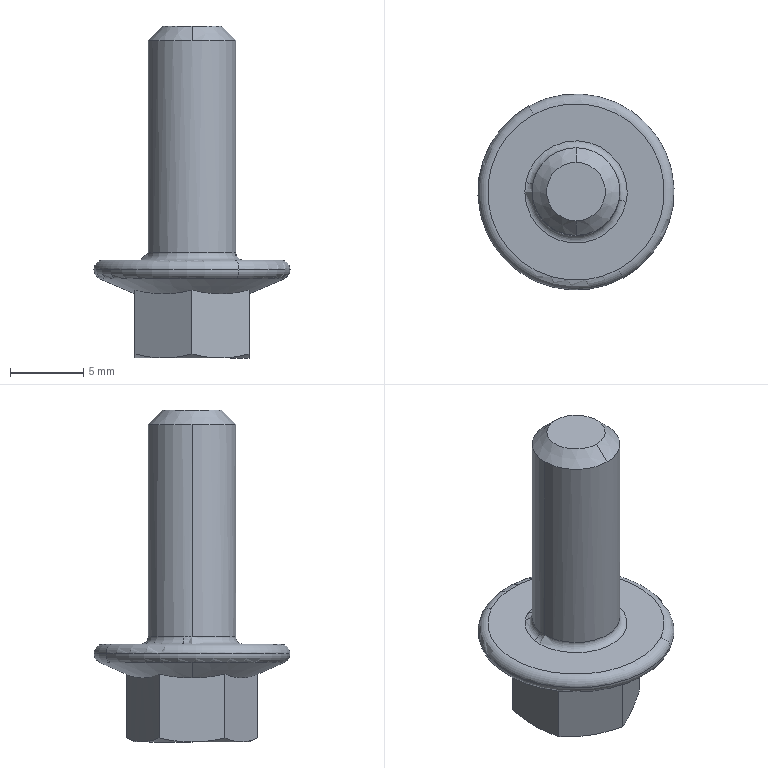Part | STEP file | M6X16_GB5787_VD-SYL0380DJ1006_1 | 1 solid | 30 faces | box 13.413 x 13.413 x 22.7 mm | volume 929.946 mm3 | cone 10 | plane 10 | torus 6 | cylinder 4 | commonest cylinder face diameters 6 x2 6.4 x2
STEP:
#1=CARTESIAN_POINT('',(0.,2.,22.7));
#2=VERTEX_POINT('',#1);
#3=CARTESIAN_POINT('',(0.,-2.,22.7));
#4=VERTEX_POINT('',#3);
#5=CARTESIAN_POINT('',(0.,0.,22.7));
#6=DIRECTION('',(0.,0.,1.));
#7=DIRECTION('',(0.,1.,0.));
#8=AXIS2_PLACEMENT_3D('',#5,#6,#7);
#9=CIRCLE('',#8,2.);
#10=EDGE_CURVE('',#2,#4,#9,.T.);
#11=ORIENTED_EDGE('',*,*,#10,.F.);
#12=CARTESIAN_POINT('',(0.,3.,21.7));
#13=VERTEX_POINT('',#12);
#14=CARTESIAN_POINT('',(0.,3.,21.7));
#15=DIRECTION('',(0.,-0.7071,0.7071));
#16=VECTOR('',#15,1000.);
#17=LINE('',#14,#16);
#18=EDGE_CURVE('',#13,#2,#17,.T.);
#19=ORIENTED_EDGE('',*,*,#18,.F.);
#20=CARTESIAN_POINT('',(-3.,0.,21.7));
#21=VERTEX_POINT('',#20);
#22=CARTESIAN_POINT('',(0.,0.,21.7));
#23=DIRECTION('',(0.,0.,1.));
#24=DIRECTION('',(0.,1.,0.));
#25=AXIS2_PLACEMENT_3D('',#22,#23,#24);
#26=CIRCLE('',#25,3.);
#27=EDGE_CURVE('',#13,#21,#26,.T.);
#28=ORIENTED_EDGE('',*,*,#27,.T.);
#29=CARTESIAN_POINT('',(0.,-3.,21.7));
#30=VERTEX_POINT('',#29);
#31=CARTESIAN_POINT('',(0.,0.,21.7));
#32=DIRECTION('',(0.,0.,1.));
#33=DIRECTION('',(-1.,0.,0.));
#34=AXIS2_PLACEMENT_3D('',#31,#32,#33);
#35=CIRCLE('',#34,3.);
#36=EDGE_CURVE('',#21,#30,#35,.T.);
#37=ORIENTED_EDGE('',*,*,#36,.T.);
#38=CARTESIAN_POINT('',(0.,-3.,21.7));
#39=DIRECTION('',(0.,0.7071,0.7071));
#40=VECTOR('',#39,1000.);
#41=LINE('',#38,#40);
#42=EDGE_CURVE('',#30,#4,#41,.T.);
#43=ORIENTED_EDGE('',*,*,#42,.T.);
#44=EDGE_LOOP('',(#11,#19,#28,#37,#43));
#45=FACE_OUTER_BOUND('',#44,.T.);
#46=CARTESIAN_POINT('',(0.,0.,22.2));
#47=DIRECTION('',(0.,0.,-1.));
#48=DIRECTION('',(0.,1.,0.));
#49=AXIS2_PLACEMENT_3D('',#46,#47,#48);
#50=CONICAL_SURFACE('',#49,2.5,0.7854);
#51=ADVANCED_FACE('',(#45),#50,.T.);
#52=ORIENTED_EDGE('',*,*,#10,.T.);
#53=CARTESIAN_POINT('',(0.,0.,22.7));
#54=DIRECTION('',(0.,0.,1.));
#55=DIRECTION('',(0.,-1.,0.));
#56=AXIS2_PLACEMENT_3D('',#53,#54,#55);
#57=CIRCLE('',#56,2.);
#58=EDGE_CURVE('',#4,#2,#57,.T.);
#59=ORIENTED_EDGE('',*,*,#58,.T.);
#60=EDGE_LOOP('',(#52,#59));
#61=FACE_OUTER_BOUND('',#60,.T.);
#62=CARTESIAN_POINT('',(0.,0.,22.7));
#63=DIRECTION('',(0.,0.,1.));
#64=DIRECTION('',(1.,0.,0.));
#65=AXIS2_PLACEMENT_3D('',#62,#63,#64);
#66=PLANE('',#65);
#67=ADVANCED_FACE('',(#61),#66,.T.);
#68=ORIENTED_EDGE('',*,*,#42,.F.);
#69=CARTESIAN_POINT('',(3.,0.,21.7));
#70=VERTEX_POINT('',#69);
#71=CARTESIAN_POINT('',(0.,0.,21.7));
#72=DIRECTION('',(0.,0.,1.));
#73=DIRECTION('',(0.,-1.,0.));
#74=AXIS2_PLACEMENT_3D('',#71,#72,#73);
#75=CIRCLE('',#74,3.);
#76=EDGE_CURVE('',#30,#70,#75,.T.);
#77=ORIENTED_EDGE('',*,*,#76,.T.);
#78=CARTESIAN_POINT('',(0.,0.,21.7));
#79=DIRECTION('',(0.,0.,1.));
#80=DIRECTION('',(1.,0.,0.));
#81=AXIS2_PLACEMENT_3D('',#78,#79,#80);
#82=CIRCLE('',#81,3.);
#83=EDGE_CURVE('',#70,#13,#82,.T.);
#84=ORIENTED_EDGE('',*,*,#83,.T.);
#85=ORIENTED_EDGE('',*,*,#18,.T.);
#86=ORIENTED_EDGE('',*,*,#58,.F.);
#87=EDGE_LOOP('',(#68,#77,#84,#85,#86));
#88=FACE_OUTER_BOUND('',#87,.T.);
#89=CARTESIAN_POINT('',(0.,0.,22.2));
#90=DIRECTION('',(0.,0.,-1.));
#91=DIRECTION('',(0.,1.,0.));
#92=AXIS2_PLACEMENT_3D('',#89,#90,#91);
#93=CONICAL_SURFACE('',#92,2.5,0.7854);
#94=ADVANCED_FACE('',(#88),#93,.T.);
#95=CARTESIAN_POINT('',(-3.,0.,7.2));
#96=VERTEX_POINT('',#95);
#97=CARTESIAN_POINT('',(-2.948,0.5558,7.2));
#98=VERTEX_POINT('',#97);
#99=CARTESIAN_POINT('',(0.,0.,7.2));
#100=DIRECTION('',(0.,0.,-1.));
#101=DIRECTION('',(-1.,0.,0.));
#102=AXIS2_PLACEMENT_3D('',#99,#100,#101);
#103=CIRCLE('',#102,3.);
#104=EDGE_CURVE('',#96,#98,#103,.T.);
#105=ORIENTED_EDGE('',*,*,#104,.F.);
#106=CARTESIAN_POINT('',(-3.,0.,21.7));
#107=DIRECTION('',(0.,0.,-1.));
#108=VECTOR('',#107,1000.);
#109=LINE('',#106,#108);
#110=EDGE_CURVE('',#21,#96,#109,.T.);
#111=ORIENTED_EDGE('',*,*,#110,.F.);
#112=ORIENTED_EDGE('',*,*,#27,.F.);
#113=ORIENTED_EDGE('',*,*,#83,.F.);
#114=CARTESIAN_POINT('',(3.,-0.000000021,7.2));
#115=VERTEX_POINT('',#114);
#116=CARTESIAN_POINT('',(3.,0.,21.7));
#117=DIRECTION('',(0.,-0.000000001,-1.));
#118=VECTOR('',#117,1000.);
#119=LINE('',#116,#118);
#120=EDGE_CURVE('',#70,#115,#119,.T.);
#121=ORIENTED_EDGE('',*,*,#120,.T.);
#122=CARTESIAN_POINT('',(0.,0.,7.2));
#123=DIRECTION('',(0.,0.,-1.));
#124=DIRECTION('',(-0.9827,0.1853,0.));
#125=AXIS2_PLACEMENT_3D('',#122,#123,#124);
#126=CIRCLE('',#125,3.);
#127=EDGE_CURVE('',#98,#115,#126,.T.);
#128=ORIENTED_EDGE('',*,*,#127,.F.);
#129=EDGE_LOOP('',(#105,#111,#112,#113,#121,#128));
#130=FACE_OUTER_BOUND('',#129,.T.);
#131=CARTESIAN_POINT('',(0.,0.,14.7));
#132=DIRECTION('',(0.,0.,1.));
#133=DIRECTION('',(1.,0.,0.));
#134=AXIS2_PLACEMENT_3D('',#131,#132,#133);
#135=CYLINDRICAL_SURFACE('',#134,3.);
#136=ADVANCED_FACE('',(#130),#135,.T.);
#137=CARTESIAN_POINT('',(2.948,-0.5558,7.2));
#138=VERTEX_POINT('',#137);
#139=CARTESIAN_POINT('',(0.,0.,7.2));
#140=DIRECTION('',(0.,0.,-1.));
#141=DIRECTION('',(0.9827,-0.1853,0.));
#142=AXIS2_PLACEMENT_3D('',#139,#140,#141);
#143=CIRCLE('',#142,3.);
#144=EDGE_CURVE('',#138,#96,#143,.T.);
#145=ORIENTED_EDGE('',*,*,#144,.F.);
#146=CARTESIAN_POINT('',(0.,0.,7.2));
#147=DIRECTION('',(0.,0.,-1.));
#148=DIRECTION('',(1.,0.,0.));
#149=AXIS2_PLACEMENT_3D('',#146,#147,#148);
#150=CIRCLE('',#149,3.);
#151=EDGE_CURVE('',#115,#138,#150,.T.);
#152=ORIENTED_EDGE('',*,*,#151,.F.);
#153=ORIENTED_EDGE('',*,*,#120,.F.);
#154=ORIENTED_EDGE('',*,*,#76,.F.);
#155=ORIENTED_EDGE('',*,*,#36,.F.);
#156=ORIENTED_EDGE('',*,*,#110,.T.);
#157=EDGE_LOOP('',(#145,#152,#153,#154,#155,#156));
#158=FACE_OUTER_BOUND('',#157,.T.);
#159=CARTESIAN_POINT('',(0.,0.,14.7));
#160=DIRECTION('',(0.,0.,1.));
#161=DIRECTION('',(1.,0.,0.));
#162=AXIS2_PLACEMENT_3D('',#159,#160,#161);
#163=CYLINDRICAL_SURFACE('',#162,3.);
#164=ADVANCED_FACE('',(#158),#163,.T.);
#165=CARTESIAN_POINT('',(3.5,-0.000000002,6.7));
#166=VERTEX_POINT('',#165);
#167=CARTESIAN_POINT('',(3.44,-0.6485,6.7));
#168=VERTEX_POINT('',#167);
#169=CARTESIAN_POINT('',(0.,0.,6.7));
#170=DIRECTION('',(0.,0.,-1.));
#171=DIRECTION('',(1.,-0.000000001,0.));
#172=AXIS2_PLACEMENT_3D('',#169,#170,#171);
#173=CIRCLE('',#172,3.5);
#174=EDGE_CURVE('',#166,#168,#173,.T.);
#175=ORIENTED_EDGE('',*,*,#174,.F.);
#176=CARTESIAN_POINT('',(-3.44,0.6486,6.7));
#177=VERTEX_POINT('',#176);
#178=CARTESIAN_POINT('',(-3.44,0.6486,6.7));
#179=CARTESIAN_POINT('',(-3.422,0.7453,6.7));
#180=CARTESIAN_POINT('',(-3.377,0.938,6.7));
#181=CARTESIAN_POINT('',(-3.279,1.238,6.7));
#182=CARTESIAN_POINT('',(-3.163,1.509,6.7));
#183=CARTESIAN_POINT('',(-3.015,1.786,6.7));
#184=CARTESIAN_POINT('',(-2.853,2.035,6.7));
#185=CARTESIAN_POINT('',(-2.662,2.28,6.7));
#186=CARTESIAN_POINT('',(-2.458,2.498,6.7));
#187=CARTESIAN_POINT('',(-2.231,2.703,6.7));
#188=CARTESIAN_POINT('',(-1.987,2.887,6.7));
#189=CARTESIAN_POINT('',(-1.729,3.048,6.7));
#190=CARTESIAN_POINT('',(-1.454,3.189,6.7));
#191=CARTESIAN_POINT('',(-1.175,3.302,6.7));
#192=CARTESIAN_POINT('',(-0.8769,3.393,6.7));
#193=CARTESIAN_POINT('',(-0.5858,3.455,6.7));
#194=CARTESIAN_POINT('',(-0.2737,3.494,6.7));
#195=CARTESIAN_POINT('',(0.01997,3.505,6.7));
#196=CARTESIAN_POINT('',(0.3356,3.489,6.7));
#197=CARTESIAN_POINT('',(0.6287,3.447,6.7));
#198=CARTESIAN_POINT('',(0.9173,3.383,6.7));
#199=CARTESIAN_POINT('',(1.218,3.286,6.7));
#200=CARTESIAN_POINT('',(1.488,3.173,6.7));
#201=CARTESIAN_POINT('',(1.766,3.027,6.7));
#202=CARTESIAN_POINT('',(2.016,2.867,6.7));
#203=CARTESIAN_POINT('',(2.262,2.677,6.7));
#204=CARTESIAN_POINT('',(2.483,2.474,6.7));
#205=CARTESIAN_POINT('',(2.69,2.246,6.7));
#206=CARTESIAN_POINT('',(2.873,2.006,6.7));
#207=CARTESIAN_POINT('',(3.035,1.752,6.7));
#208=CARTESIAN_POINT('',(3.178,1.478,6.7));
#209=CARTESIAN_POINT('',(3.293,1.2,6.7));
#210=CARTESIAN_POINT('',(3.387,0.9026,6.7));
#211=CARTESIAN_POINT('',(3.451,0.611,6.7));
#212=CARTESIAN_POINT('',(3.492,0.2996,6.7));
#213=CARTESIAN_POINT('',(3.5,0.09972,6.7));
#214=CARTESIAN_POINT('',(3.5,-0.000000002,6.7));
#215=B_SPLINE_CURVE_WITH_KNOTS('',3,(#178,#179,#180,#181,#182,#183,#184,#185,#186,#187,#188,#189,#190,#191,#192,#193,#194,#195,#196,#197,#198,#199,#200,#201,#202,#203,#204,#205,#206,#207,#208,#209,#210,#211,#212,#213,#214),.UNSPECIFIED.,.F.,.F.,(4,1,1,1,1,1,1,1,1,1,1,1,1,1,1,1,1,1,1,1,1,1,1,1,1,1,1,1,1,1,1,1,1,1,4),(0.,0.02941,0.05882,0.08824,0.1176,0.1471,0.1765,0.2059,0.2353,0.2647,0.2941,0.3235,0.3529,0.3824,0.4118,0.4412,0.4706,0.5,0.5294,0.5588,0.5882,0.6176,0.6471,0.6765,0.7059,0.7353,0.7647,0.7941,0.8235,0.8529,0.8824,0.9118,0.9412,0.9706,1.),.UNSPECIFIED.);
#216=EDGE_CURVE('',#177,#166,#215,.T.);
#217=ORIENTED_EDGE('',*,*,#216,.F.);
#218=CARTESIAN_POINT('',(-3.439,0.6485,7.2));
#219=DIRECTION('',(0.1853,0.9827,0.));
#220=DIRECTION('',(0.9827,-0.1853,0.));
#221=AXIS2_PLACEMENT_3D('',#218,#219,#220);
#222=CIRCLE('',#221,0.5);
#223=EDGE_CURVE('',#98,#177,#222,.T.);
#224=ORIENTED_EDGE('',*,*,#223,.F.);
#225=ORIENTED_EDGE('',*,*,#127,.T.);
#226=ORIENTED_EDGE('',*,*,#151,.T.);
#227=CARTESIAN_POINT('',(3.439,-0.6485,7.2));
#228=DIRECTION('',(-0.1853,-0.9827,0.));
#229=DIRECTION('',(-0.9827,0.1853,0.));
#230=AXIS2_PLACEMENT_3D('',#227,#228,#229);
#231=CIRCLE('',#230,0.5);
#232=EDGE_CURVE('',#138,#168,#231,.T.);
#233=ORIENTED_EDGE('',*,*,#232,.T.);
#234=EDGE_LOOP('',(#175,#217,#224,#225,#226,#233));
#235=FACE_OUTER_BOUND('',#234,.T.);
#236=CARTESIAN_POINT('',(0.,0.,7.2));
#237=DIRECTION('',(0.,0.,1.));
#238=DIRECTION('',(0.9827,-0.1853,0.));
#239=AXIS2_PLACEMENT_3D('',#236,#237,#238);
#240=TOROIDAL_SURFACE('',#239,3.5,0.5);
#241=ADVANCED_FACE('',(#235),#240,.F.);
#242=CARTESIAN_POINT('',(-3.2,0.,0.2));
#243=VERTEX_POINT('',#242);
#244=CARTESIAN_POINT('',(3.2,0.,0.2));
#245=VERTEX_POINT('',#244);
#246=CARTESIAN_POINT('',(0.,0.,0.2));
#247=DIRECTION('',(0.,0.,-1.));
#248=DIRECTION('',(-1.,0.,0.));
#249=AXIS2_PLACEMENT_3D('',#246,#247,#248);
#250=CIRCLE('',#249,3.2);
#251=EDGE_CURVE('',#243,#245,#250,.T.);
#252=ORIENTED_EDGE('',*,*,#251,.T.);
#253=CARTESIAN_POINT('',(0.,0.,0.2));
#254=DIRECTION('',(0.,0.,-1.));
#255=DIRECTION('',(1.,0.,0.));
#256=AXIS2_PLACEMENT_3D('',#253,#254,#255);
#257=CIRCLE('',#256,3.2);
#258=EDGE_CURVE('',#245,#243,#257,.T.);
#259=ORIENTED_EDGE('',*,*,#258,.T.);
#260=EDGE_LOOP('',(#252,#259));
#261=FACE_OUTER_BOUND('',#260,.T.);
#262=CARTESIAN_POINT('',(0.,0.,0.2));
#263=DIRECTION('',(0.,0.,1.));
#264=DIRECTION('',(1.,0.,0.));
#265=AXIS2_PLACEMENT_3D('',#262,#263,#264);
#266=PLANE('',#265);
#267=ADVANCED_FACE('',(#261),#266,.F.);
#268=CARTESIAN_POINT('',(3.2,0.,0.));
#269=VERTEX_POINT('',#268);
#270=CARTESIAN_POINT('',(-3.2,0.,0.));
#271=VERTEX_POINT('',#270);
#272=CARTESIAN_POINT('',(0.,0.,0.));
#273=DIRECTION('',(0.,0.,1.));
#274=DIRECTION('',(1.,0.,0.));
#275=AXIS2_PLACEMENT_3D('',#272,#273,#274);
#276=CIRCLE('',#275,3.2);
#277=EDGE_CURVE('',#269,#271,#276,.T.);
#278=ORIENTED_EDGE('',*,*,#277,.F.);
#279=CARTESIAN_POINT('',(3.2,0.,0.2));
#280=DIRECTION('',(0.,0.,-1.));
#281=VECTOR('',#280,1000.);
#282=LINE('',#279,#281);
#283=EDGE_CURVE('',#245,#269,#282,.T.);
#284=ORIENTED_EDGE('',*,*,#283,.F.);
#285=ORIENTED_EDGE('',*,*,#251,.F.);
#286=CARTESIAN_POINT('',(-3.2,0.,0.2));
#287=DIRECTION('',(0.,0.,-1.));
#288=VECTOR('',#287,1000.);
#289=LINE('',#286,#288);
#290=EDGE_CURVE('',#243,#271,#289,.T.);
#291=ORIENTED_EDGE('',*,*,#290,.T.);
#292=EDGE_LOOP('',(#278,#284,#285,#291));
#293=FACE_OUTER_BOUND('',#292,.T.);
#294=CARTESIAN_POINT('',(0.,0.,0.1));
#295=DIRECTION('',(0.,0.,1.));
#296=DIRECTION('',(1.,0.,0.));
#297=AXIS2_PLACEMENT_3D('',#294,#295,#296);
#298=CYLINDRICAL_SURFACE('',#297,3.2);
#299=ADVANCED_FACE('',(#293),#298,.F.);
#300=ORIENTED_EDGE('',*,*,#290,.F.);
#301=ORIENTED_EDGE('',*,*,#258,.F.);
#302=ORIENTED_EDGE('',*,*,#283,.T.);
#303=CARTESIAN_POINT('',(0.,0.,0.));
#304=DIRECTION('',(0.,0.,1.));
#305=DIRECTION('',(-1.,0.,0.));
#306=AXIS2_PLACEMENT_3D('',#303,#304,#305);
#307=CIRCLE('',#306,3.2);
#308=EDGE_CURVE('',#271,#269,#307,.T.);
#309=ORIENTED_EDGE('',*,*,#308,.F.);
#310=EDGE_LOOP('',(#300,#301,#302,#309));
#311=FACE_OUTER_BOUND('',#310,.T.);
#312=CARTESIAN_POINT('',(0.,0.,0.1));
#313=DIRECTION('',(0.,0.,1.));
#314=DIRECTION('',(1.,0.,0.));
#315=AXIS2_PLACEMENT_3D('',#312,#313,#314);
#316=CYLINDRICAL_SURFACE('',#315,3.2);
#317=ADVANCED_FACE('',(#311),#316,.F.);
#318=CARTESIAN_POINT('',(1.95,-3.377,0.000000001));
#319=VERTEX_POINT('',#318);
#320=CARTESIAN_POINT('',(-1.95,-3.377,0.));
#321=VERTEX_POINT('',#320);
#322=CARTESIAN_POINT('',(0.,0.,0.000000001));
#323=DIRECTION('',(0.,0.,-1.));
#324=DIRECTION('',(0.5,-0.866,0.));
#325=AXIS2_PLACEMENT_3D('',#322,#323,#324);
#326=CIRCLE('',#325,3.9);
#327=EDGE_CURVE('',#319,#321,#326,.T.);
#328=ORIENTED_EDGE('',*,*,#327,.F.);
#329=CARTESIAN_POINT('',(0.,-4.503,0.2813));
#330=VERTEX_POINT('',#329);
#331=CARTESIAN_POINT('',(1.95,-3.377,0.000000001));
#332=CARTESIAN_POINT('',(1.789,-3.471,0.000000001));
#333=CARTESIAN_POINT('',(1.629,-3.562,0.006075));
#334=CARTESIAN_POINT('',(1.39,-3.701,0.0243));
#335=CARTESIAN_POINT('',(1.309,-3.747,0.03189));
#336=CARTESIAN_POINT('',(1.148,-3.841,0.05012));
#337=CARTESIAN_POINT('',(1.065,-3.889,0.06103));
#338=CARTESIAN_POINT('',(0.663,-4.12,0.1204));
#339=CARTESIAN_POINT('',(0.3398,-4.307,0.1898));
#340=CARTESIAN_POINT('',(0.,-4.503,0.2813));
#341=B_SPLINE_CURVE_WITH_KNOTS('',3,(#331,#332,#333,#334,#335,#336,#337,#338,#339,#340),.UNSPECIFIED.,.F.,.F.,(4,2,2,2,4),(0.,0.25,0.375,0.5,1.),.UNSPECIFIED.);
#342=EDGE_CURVE('',#319,#330,#341,.T.);
#343=ORIENTED_EDGE('',*,*,#342,.T.);
#344=CARTESIAN_POINT('',(0.,-4.503,0.2813));
#345=CARTESIAN_POINT('',(-0.17,-4.405,0.2356));
#346=CARTESIAN_POINT('',(-0.3359,-4.309,0.1953));
#347=CARTESIAN_POINT('',(-0.5813,-4.168,0.1432));
#348=CARTESIAN_POINT('',(-0.6625,-4.121,0.1272));
#349=CARTESIAN_POINT('',(-0.8241,-4.027,0.09792));
#350=CARTESIAN_POINT('',(-0.9029,-3.982,0.08494));
#351=CARTESIAN_POINT('',(-1.314,-3.745,0.02427));
#352=CARTESIAN_POINT('',(-1.627,-3.564,0.));
#353=CARTESIAN_POINT('',(-1.95,-3.377,0.));
#354=B_SPLINE_CURVE_WITH_KNOTS('',3,(#344,#345,#346,#347,#348,#349,#350,#351,#352,#353),.UNSPECIFIED.,.F.,.F.,(4,2,2,2,4),(0.,0.25,0.375,0.5,1.),.UNSPECIFIED.);
#355=EDGE_CURVE('',#330,#321,#354,.T.);
#356=ORIENTED_EDGE('',*,*,#355,.T.);
#357=EDGE_LOOP('',(#328,#343,#356));
#358=FACE_OUTER_BOUND('',#357,.T.);
#359=CARTESIAN_POINT('',(0.,0.,0.1407));
#360=DIRECTION('',(0.,0.,1.));
#361=DIRECTION('',(1.,0.,0.));
#362=AXIS2_PLACEMENT_3D('',#359,#360,#361);
#363=CONICAL_SURFACE('',#362,4.202,1.134);
#364=ADVANCED_FACE('',(#358),#363,.T.);
#365=CARTESIAN_POINT('',(-3.9,-2.131,0.2537));
#366=VERTEX_POINT('',#365);
#367=CARTESIAN_POINT('',(-3.9,-0.000000014,0.));
#368=VERTEX_POINT('',#367);
#369=CARTESIAN_POINT('',(-3.9,-2.131,0.2537));
#370=CARTESIAN_POINT('',(-3.9,-1.946,0.2124));
#371=CARTESIAN_POINT('',(-3.9,-1.765,0.176));
#372=CARTESIAN_POINT('',(-3.9,-1.497,0.129));
#373=CARTESIAN_POINT('',(-3.9,-1.409,0.1145));
#374=CARTESIAN_POINT('',(-3.9,-1.232,0.08815));
#375=CARTESIAN_POINT('',(-3.9,-1.146,0.07642));
#376=CARTESIAN_POINT('',(-3.9,-0.697,0.02183));
#377=CARTESIAN_POINT('',(-3.9,-0.353,0.));
#378=CARTESIAN_POINT('',(-3.9,-0.000000014,0.));
#379=B_SPLINE_CURVE_WITH_KNOTS('',3,(#369,#370,#371,#372,#373,#374,#375,#376,#377,#378),.UNSPECIFIED.,.F.,.F.,(4,2,2,2,4),(0.,0.25,0.375,0.5,1.),.UNSPECIFIED.);
#380=EDGE_CURVE('',#366,#368,#379,.T.);
#381=ORIENTED_EDGE('',*,*,#380,.T.);
#382=CARTESIAN_POINT('',(0.,0.,0.));
#383=DIRECTION('',(0.,0.,-1.));
#384=DIRECTION('',(-0.5,-0.866,0.));
#385=AXIS2_PLACEMENT_3D('',#382,#383,#384);
#386=CIRCLE('',#385,3.9);
#387=EDGE_CURVE('',#321,#368,#386,.T.);
#388=ORIENTED_EDGE('',*,*,#387,.F.);
#389=CARTESIAN_POINT('',(-3.9,-2.252,0.2813));
#390=VERTEX_POINT('',#389);
#391=CARTESIAN_POINT('',(-1.95,-3.377,0.));
#392=CARTESIAN_POINT('',(-2.111,-3.284,0.));
#393=CARTESIAN_POINT('',(-2.27,-3.192,0.006075));
#394=CARTESIAN_POINT('',(-2.51,-3.054,0.0243));
#395=CARTESIAN_POINT('',(-2.591,-3.008,0.03189));
#396=CARTESIAN_POINT('',(-2.752,-2.914,0.05012));
#397=CARTESIAN_POINT('',(-2.835,-2.866,0.06103));
#398=CARTESIAN_POINT('',(-3.237,-2.634,0.1204));
#399=CARTESIAN_POINT('',(-3.56,-2.448,0.1898));
#400=CARTESIAN_POINT('',(-3.9,-2.252,0.2813));
#401=B_SPLINE_CURVE_WITH_KNOTS('',3,(#391,#392,#393,#394,#395,#396,#397,#398,#399,#400),.UNSPECIFIED.,.F.,.F.,(4,2,2,2,4),(0.,0.25,0.375,0.5,1.),.UNSPECIFIED.);
#402=EDGE_CURVE('',#321,#390,#401,.T.);
#403=ORIENTED_EDGE('',*,*,#402,.T.);
#404=CARTESIAN_POINT('',(-3.9,-2.252,0.2813));
#405=CARTESIAN_POINT('',(-3.9,-2.238,0.2782));
#406=CARTESIAN_POINT('',(-3.9,-2.211,0.272));
#407=CARTESIAN_POINT('',(-3.9,-2.171,0.2627));
#408=CARTESIAN_POINT('',(-3.9,-2.144,0.2567));
#409=CARTESIAN_POINT('',(-3.9,-2.131,0.2537));
#410=B_SPLINE_CURVE_WITH_KNOTS('',3,(#404,#405,#406,#407,#408,#409),.UNSPECIFIED.,.F.,.F.,(4,1,1,4),(0.,0.3333,0.6667,1.),.UNSPECIFIED.);
#411=EDGE_CURVE('',#390,#366,#410,.T.);
#412=ORIENTED_EDGE('',*,*,#411,.T.);
#413=EDGE_LOOP('',(#381,#388,#403,#412));
#414=FACE_OUTER_BOUND('',#413,.T.);
#415=CARTESIAN_POINT('',(0.,0.,0.1407));
#416=DIRECTION('',(0.,0.,1.));
#417=DIRECTION('',(1.,0.,0.));
#418=AXIS2_PLACEMENT_3D('',#415,#416,#417);
#419=CONICAL_SURFACE('',#418,4.202,1.134);
#420=ADVANCED_FACE('',(#414),#419,.T.);
#421=CARTESIAN_POINT('',(-1.95,3.377,0.));
#422=VERTEX_POINT('',#421);
#423=CARTESIAN_POINT('',(1.95,3.377,0.));
#424=VERTEX_POINT('',#423);
#425=CARTESIAN_POINT('',(0.,0.,0.));
#426=DIRECTION('',(0.,0.,-1.));
#427=DIRECTION('',(-0.5,0.866,0.));
#428=AXIS2_PLACEMENT_3D('',#425,#426,#427);
#429=CIRCLE('',#428,3.9);
#430=EDGE_CURVE('',#422,#424,#429,.T.);
#431=ORIENTED_EDGE('',*,*,#430,.F.);
#432=CARTESIAN_POINT('',(0.,4.503,0.2813));
#433=VERTEX_POINT('',#432);
#434=CARTESIAN_POINT('',(-1.95,3.377,0.));
#435=CARTESIAN_POINT('',(-1.789,3.471,0.));
#436=CARTESIAN_POINT('',(-1.629,3.562,0.006075));
#437=CARTESIAN_POINT('',(-1.39,3.701,0.0243));
#438=CARTESIAN_POINT('',(-1.309,3.747,0.03189));
#439=CARTESIAN_POINT('',(-1.148,3.841,0.05012));
#440=CARTESIAN_POINT('',(-1.065,3.889,0.06103));
#441=CARTESIAN_POINT('',(-0.663,4.12,0.1204));
#442=CARTESIAN_POINT('',(-0.3398,4.307,0.1898));
#443=CARTESIAN_POINT('',(0.,4.503,0.2813));
#444=B_SPLINE_CURVE_WITH_KNOTS('',3,(#434,#435,#436,#437,#438,#439,#440,#441,#442,#443),.UNSPECIFIED.,.F.,.F.,(4,2,2,2,4),(0.,0.25,0.375,0.5,1.),.UNSPECIFIED.);
#445=EDGE_CURVE('',#422,#433,#444,.T.);
#446=ORIENTED_EDGE('',*,*,#445,.T.);
#447=CARTESIAN_POINT('',(0.,4.503,0.2813));
#448=CARTESIAN_POINT('',(0.17,4.405,0.2356));
#449=CARTESIAN_POINT('',(0.3359,4.309,0.1953));
#450=CARTESIAN_POINT('',(0.5813,4.168,0.1432));
#451=CARTESIAN_POINT('',(0.6625,4.121,0.1272));
#452=CARTESIAN_POINT('',(0.8241,4.027,0.09792));
#453=CARTESIAN_POINT('',(0.9029,3.982,0.08494));
#454=CARTESIAN_POINT('',(1.314,3.745,0.02427));
#455=CARTESIAN_POINT('',(1.627,3.564,0.));
#456=CARTESIAN_POINT('',(1.95,3.377,0.));
#457=B_SPLINE_CURVE_WITH_KNOTS('',3,(#447,#448,#449,#450,#451,#452,#453,#454,#455,#456),.UNSPECIFIED.,.F.,.F.,(4,2,2,2,4),(0.,0.25,0.375,0.5,1.),.UNSPECIFIED.);
#458=EDGE_CURVE('',#433,#424,#457,.T.);
#459=ORIENTED_EDGE('',*,*,#458,.T.);
#460=EDGE_LOOP('',(#431,#446,#459));
#461=FACE_OUTER_BOUND('',#460,.T.);
#462=CARTESIAN_POINT('',(0.,0.,0.1407));
#463=DIRECTION('',(0.,0.,1.));
#464=DIRECTION('',(1.,0.,0.));
#465=AXIS2_PLACEMENT_3D('',#462,#463,#464);
#466=CONICAL_SURFACE('',#465,4.202,1.134);
#467=ADVANCED_FACE('',(#461),#466,.T.);
#468=CARTESIAN_POINT('',(3.9,-0.000000011,0.));
#469=VERTEX_POINT('',#468);
#470=CARTESIAN_POINT('',(0.,0.,0.));
#471=DIRECTION('',(0.,0.,-1.));
#472=DIRECTION('',(0.5,0.866,0.));
#473=AXIS2_PLACEMENT_3D('',#470,#471,#472);
#474=CIRCLE('',#473,3.9);
#475=EDGE_CURVE('',#424,#469,#474,.T.);
#476=ORIENTED_EDGE('',*,*,#475,.F.);
#477=CARTESIAN_POINT('',(3.9,2.252,0.2813));
#478=VERTEX_POINT('',#477);
#479=CARTESIAN_POINT('',(1.95,3.377,0.));
#480=CARTESIAN_POINT('',(2.111,3.284,0.));
#481=CARTESIAN_POINT('',(2.27,3.192,0.006075));
#482=CARTESIAN_POINT('',(2.51,3.054,0.0243));
#483=CARTESIAN_POINT('',(2.591,3.008,0.03189));
#484=CARTESIAN_POINT('',(2.752,2.914,0.05012));
#485=CARTESIAN_POINT('',(2.835,2.866,0.06103));
#486=CARTESIAN_POINT('',(3.237,2.634,0.1204));
#487=CARTESIAN_POINT('',(3.56,2.448,0.1898));
#488=CARTESIAN_POINT('',(3.9,2.252,0.2813));
#489=B_SPLINE_CURVE_WITH_KNOTS('',3,(#479,#480,#481,#482,#483,#484,#485,#486,#487,#488),.UNSPECIFIED.,.F.,.F.,(4,2,2,2,4),(0.,0.25,0.375,0.5,1.),.UNSPECIFIED.);
#490=EDGE_CURVE('',#424,#478,#489,.T.);
#491=ORIENTED_EDGE('',*,*,#490,.T.);
#492=CARTESIAN_POINT('',(3.9,2.252,0.2813));
#493=CARTESIAN_POINT('',(3.9,2.055,0.2356));
#494=CARTESIAN_POINT('',(3.9,1.864,0.1953));
#495=CARTESIAN_POINT('',(3.9,1.58,0.1432));
#496=CARTESIAN_POINT('',(3.9,1.487,0.1272));
#497=CARTESIAN_POINT('',(3.9,1.3,0.09792));
#498=CARTESIAN_POINT('',(3.9,1.209,0.08494));
#499=CARTESIAN_POINT('',(3.9,0.7347,0.02427));
#500=CARTESIAN_POINT('',(3.9,0.3726,0.));
#501=CARTESIAN_POINT('',(3.9,-0.000000011,0.));
#502=B_SPLINE_CURVE_WITH_KNOTS('',3,(#492,#493,#494,#495,#496,#497,#498,#499,#500,#501),.UNSPECIFIED.,.F.,.F.,(4,2,2,2,4),(0.,0.25,0.375,0.5,1.),.UNSPECIFIED.);
#503=EDGE_CURVE('',#478,#469,#502,.T.);
#504=ORIENTED_EDGE('',*,*,#503,.T.);
#505=EDGE_LOOP('',(#476,#491,#504));
#506=FACE_OUTER_BOUND('',#505,.T.);
#507=CARTESIAN_POINT('',(0.,0.,0.1407));
#508=DIRECTION('',(0.,0.,1.));
#509=DIRECTION('',(1.,0.,0.));
#510=AXIS2_PLACEMENT_3D('',#507,#508,#509);
#511=CONICAL_SURFACE('',#510,4.202,1.134);
#512=ADVANCED_FACE('',(#506),#511,.T.);
#513=CARTESIAN_POINT('',(0.,0.,0.000000001));
#514=DIRECTION('',(0.,0.,-1.));
#515=DIRECTION('',(1.,-0.000000003,0.));
#516=AXIS2_PLACEMENT_3D('',#513,#514,#515);
#517=CIRCLE('',#516,3.9);
#518=EDGE_CURVE('',#469,#319,#517,.T.);
#519=ORIENTED_EDGE('',*,*,#518,.F.);
#520=CARTESIAN_POINT('',(3.9,-2.252,0.2813));
#521=VERTEX_POINT('',#520);
#522=CARTESIAN_POINT('',(3.9,-0.000000011,0.));
#523=CARTESIAN_POINT('',(3.9,-0.1864,0.));
#524=CARTESIAN_POINT('',(3.9,-0.3701,0.006075));
#525=CARTESIAN_POINT('',(3.9,-0.6471,0.0243));
#526=CARTESIAN_POINT('',(3.9,-0.7397,0.03189));
#527=CARTESIAN_POINT('',(3.9,-0.9261,0.05012));
#528=CARTESIAN_POINT('',(3.9,-1.022,0.06103));
#529=CARTESIAN_POINT('',(3.9,-1.486,0.1204));
#530=CARTESIAN_POINT('',(3.9,-1.859,0.1898));
#531=CARTESIAN_POINT('',(3.9,-2.252,0.2813));
#532=B_SPLINE_CURVE_WITH_KNOTS('',3,(#522,#523,#524,#525,#526,#527,#528,#529,#530,#531),.UNSPECIFIED.,.F.,.F.,(4,2,2,2,4),(0.,0.25,0.375,0.5,1.),.UNSPECIFIED.);
#533=EDGE_CURVE('',#469,#521,#532,.T.);
#534=ORIENTED_EDGE('',*,*,#533,.T.);
#535=CARTESIAN_POINT('',(3.9,-2.252,0.2813));
#536=CARTESIAN_POINT('',(3.73,-2.35,0.2356));
#537=CARTESIAN_POINT('',(3.564,-2.446,0.1953));
#538=CARTESIAN_POINT('',(3.319,-2.587,0.1432));
#539=CARTESIAN_POINT('',(3.237,-2.634,0.1272));
#540=CARTESIAN_POINT('',(3.076,-2.727,0.09792));
#541=CARTESIAN_POINT('',(2.997,-2.773,0.08494));
#542=CARTESIAN_POINT('',(2.586,-3.01,0.02427));
#543=CARTESIAN_POINT('',(2.273,-3.191,0.000000001));
#544=CARTESIAN_POINT('',(1.95,-3.377,0.000000001));
#545=B_SPLINE_CURVE_WITH_KNOTS('',3,(#535,#536,#537,#538,#539,#540,#541,#542,#543,#544),.UNSPECIFIED.,.F.,.F.,(4,2,2,2,4),(0.,0.25,0.375,0.5,1.),.UNSPECIFIED.);
#546=EDGE_CURVE('',#521,#319,#545,.T.);
#547=ORIENTED_EDGE('',*,*,#546,.T.);
#548=EDGE_LOOP('',(#519,#534,#547));
#549=FACE_OUTER_BOUND('',#548,.T.);
#550=CARTESIAN_POINT('',(0.,0.,0.1407));
#551=DIRECTION('',(0.,0.,1.));
#552=DIRECTION('',(1.,0.,0.));
#553=AXIS2_PLACEMENT_3D('',#550,#551,#552);
#554=CONICAL_SURFACE('',#553,4.202,1.134);
#555=ADVANCED_FACE('',(#549),#554,.T.);
#556=ORIENTED_EDGE('',*,*,#277,.T.);
#557=ORIENTED_EDGE('',*,*,#308,.T.);
#558=EDGE_LOOP('',(#556,#557));
#559=FACE_BOUND('',#558,.T.);
#560=ORIENTED_EDGE('',*,*,#327,.T.);
#561=ORIENTED_EDGE('',*,*,#387,.T.);
#562=CARTESIAN_POINT('',(0.,0.,0.));
#563=DIRECTION('',(0.,0.,-1.));
#564=DIRECTION('',(-1.,0.,0.));
#565=AXIS2_PLACEMENT_3D('',#562,#563,#564);
#566=CIRCLE('',#565,3.9);
#567=EDGE_CURVE('',#368,#422,#566,.T.);
#568=ORIENTED_EDGE('',*,*,#567,.T.);
#569=ORIENTED_EDGE('',*,*,#430,.T.);
#570=ORIENTED_EDGE('',*,*,#475,.T.);
#571=ORIENTED_EDGE('',*,*,#518,.T.);
#572=EDGE_LOOP('',(#560,#561,#568,#569,#570,#571));
#573=FACE_OUTER_BOUND('',#572,.T.);
#574=CARTESIAN_POINT('',(0.,0.,0.));
#575=DIRECTION('',(0.,0.,1.));
#576=DIRECTION('',(1.,0.,0.));
#577=AXIS2_PLACEMENT_3D('',#574,#575,#576);
#578=PLANE('',#577);
#579=ADVANCED_FACE('',(#559,#573),#578,.F.);
#580=ORIENTED_EDGE('',*,*,#567,.F.);
#581=CARTESIAN_POINT('',(-3.9,2.252,0.2813));
#582=VERTEX_POINT('',#581);
#583=CARTESIAN_POINT('',(-3.9,-0.000000014,0.));
#584=CARTESIAN_POINT('',(-3.9,0.1864,0.));
#585=CARTESIAN_POINT('',(-3.9,0.3701,0.006075));
#586=CARTESIAN_POINT('',(-3.9,0.6471,0.0243));
#587=CARTESIAN_POINT('',(-3.9,0.7397,0.03189));
#588=CARTESIAN_POINT('',(-3.9,0.9261,0.05012));
#589=CARTESIAN_POINT('',(-3.9,1.022,0.06103));
#590=CARTESIAN_POINT('',(-3.9,1.486,0.1204));
#591=CARTESIAN_POINT('',(-3.9,1.859,0.1898));
#592=CARTESIAN_POINT('',(-3.9,2.252,0.2813));
#593=B_SPLINE_CURVE_WITH_KNOTS('',3,(#583,#584,#585,#586,#587,#588,#589,#590,#591,#592),.UNSPECIFIED.,.F.,.F.,(4,2,2,2,4),(0.,0.25,0.375,0.5,1.),.UNSPECIFIED.);
#594=EDGE_CURVE('',#368,#582,#593,.T.);
#595=ORIENTED_EDGE('',*,*,#594,.T.);
#596=CARTESIAN_POINT('',(-3.9,2.252,0.2813));
#597=CARTESIAN_POINT('',(-3.73,2.35,0.2356));
#598=CARTESIAN_POINT('',(-3.564,2.446,0.1953));
#599=CARTESIAN_POINT('',(-3.319,2.587,0.1432));
#600=CARTESIAN_POINT('',(-3.237,2.634,0.1272));
#601=CARTESIAN_POINT('',(-3.076,2.727,0.09792));
#602=CARTESIAN_POINT('',(-2.997,2.773,0.08494));
#603=CARTESIAN_POINT('',(-2.586,3.01,0.02427));
#604=CARTESIAN_POINT('',(-2.273,3.191,0.));
#605=CARTESIAN_POINT('',(-1.95,3.377,0.));
#606=B_SPLINE_CURVE_WITH_KNOTS('',3,(#596,#597,#598,#599,#600,#601,#602,#603,#604,#605),.UNSPECIFIED.,.F.,.F.,(4,2,2,2,4),(0.,0.25,0.375,0.5,1.),.UNSPECIFIED.);
#607=EDGE_CURVE('',#582,#422,#606,.T.);
#608=ORIENTED_EDGE('',*,*,#607,.T.);
#609=EDGE_LOOP('',(#580,#595,#608));
#610=FACE_OUTER_BOUND('',#609,.T.);
#611=CARTESIAN_POINT('',(0.,0.,0.1407));
#612=DIRECTION('',(0.,0.,1.));
#613=DIRECTION('',(1.,0.,0.));
#614=AXIS2_PLACEMENT_3D('',#611,#612,#613);
#615=CONICAL_SURFACE('',#614,4.202,1.134);
#616=ADVANCED_FACE('',(#610),#615,.T.);
#617=CARTESIAN_POINT('',(0.000000012,4.503,4.646));
#618=VERTEX_POINT('',#617);
#619=CARTESIAN_POINT('',(0.,4.503,0.2813));
#620=DIRECTION('',(0.000000003,0.000000002,1.));
#621=VECTOR('',#620,1000.);
#622=LINE('',#619,#621);
#623=EDGE_CURVE('',#433,#618,#622,.T.);
#624=ORIENTED_EDGE('',*,*,#623,.F.);
#625=ORIENTED_EDGE('',*,*,#445,.F.);
#626=ORIENTED_EDGE('',*,*,#607,.F.);
#627=CARTESIAN_POINT('',(-3.9,2.252,4.646));
#628=VERTEX_POINT('',#627);
#629=CARTESIAN_POINT('',(-3.9,2.252,4.646));
#630=DIRECTION('',(0.,-0.000000007,-1.));
#631=VECTOR('',#630,1000.);
#632=LINE('',#629,#631);
#633=EDGE_CURVE('',#628,#582,#632,.T.);
#634=ORIENTED_EDGE('',*,*,#633,.F.);
#635=CARTESIAN_POINT('',(0.000000012,4.503,4.646));
#636=CARTESIAN_POINT('',(-0.1679,4.406,4.604));
#637=CARTESIAN_POINT('',(-0.3319,4.312,4.568));
#638=CARTESIAN_POINT('',(-0.5746,4.171,4.52));
#639=CARTESIAN_POINT('',(-0.6549,4.125,4.506));
#640=CARTESIAN_POINT('',(-0.7749,4.056,4.485));
#641=CARTESIAN_POINT('',(-0.8148,4.033,4.479));
#642=CARTESIAN_POINT('',(-0.8945,3.987,4.467));
#643=CARTESIAN_POINT('',(-0.9326,3.965,4.461));
#644=CARTESIAN_POINT('',(-1.306,3.749,4.41));
#645=CARTESIAN_POINT('',(-1.624,3.566,4.387));
#646=CARTESIAN_POINT('',(-2.114,3.282,4.387));
#647=CARTESIAN_POINT('',(-2.275,3.189,4.393));
#648=CARTESIAN_POINT('',(-2.518,3.049,4.41));
#649=CARTESIAN_POINT('',(-2.599,3.003,4.417));
#650=CARTESIAN_POINT('',(-2.721,2.932,4.43));
#651=CARTESIAN_POINT('',(-2.762,2.908,4.435));
#652=CARTESIAN_POINT('',(-2.845,2.861,4.445));
#653=CARTESIAN_POINT('',(-2.888,2.836,4.45));
#654=CARTESIAN_POINT('',(-3.245,2.63,4.5));
#655=CARTESIAN_POINT('',(-3.565,2.445,4.563));
#656=CARTESIAN_POINT('',(-3.9,2.252,4.646));
#657=B_SPLINE_CURVE_WITH_KNOTS('',3,(#635,#636,#637,#638,#639,#640,#641,#642,#643,#644,#645,#646,#647,#648,#649,#650,#651,#652,#653,#654,#655,#656),.UNSPECIFIED.,.F.,.F.,(4,2,2,2,2,2,2,2,2,2,4),(0.,0.125,0.1875,0.2188,0.25,0.5,0.625,0.6875,0.7188,0.75,1.),.UNSPECIFIED.);
#658=EDGE_CURVE('',#618,#628,#657,.T.);
#659=ORIENTED_EDGE('',*,*,#658,.F.);
#660=EDGE_LOOP('',(#624,#625,#626,#634,#659));
#661=FACE_OUTER_BOUND('',#660,.T.);
#662=CARTESIAN_POINT('',(0.,4.503,0.));
#663=DIRECTION('',(-0.5,0.866,0.));
#664=DIRECTION('',(0.,0.,1.));
#665=AXIS2_PLACEMENT_3D('',#662,#663,#664);
#666=PLANE('',#665);
#667=ADVANCED_FACE('',(#661),#666,.T.);
#668=CARTESIAN_POINT('',(3.9,2.252,4.646));
#669=VERTEX_POINT('',#668);
#670=CARTESIAN_POINT('',(3.9,2.252,0.2813));
#671=DIRECTION('',(0.000000003,-0.000000002,1.));
#672=VECTOR('',#671,1000.);
#673=LINE('',#670,#672);
#674=EDGE_CURVE('',#478,#669,#673,.T.);
#675=ORIENTED_EDGE('',*,*,#674,.F.);
#676=ORIENTED_EDGE('',*,*,#490,.F.);
#677=ORIENTED_EDGE('',*,*,#458,.F.);
#678=ORIENTED_EDGE('',*,*,#623,.T.);
#679=CARTESIAN_POINT('',(3.9,2.252,4.646));
#680=CARTESIAN_POINT('',(3.732,2.349,4.604));
#681=CARTESIAN_POINT('',(3.567,2.444,4.568));
#682=CARTESIAN_POINT('',(3.324,2.584,4.52));
#683=CARTESIAN_POINT('',(3.243,2.631,4.505));
#684=CARTESIAN_POINT('',(3.123,2.7,4.485));
#685=CARTESIAN_POINT('',(3.083,2.723,4.479));
#686=CARTESIAN_POINT('',(3.003,2.77,4.467));
#687=CARTESIAN_POINT('',(2.965,2.792,4.461));
#688=CARTESIAN_POINT('',(2.592,3.007,4.41));
#689=CARTESIAN_POINT('',(2.275,3.19,4.387));
#690=CARTESIAN_POINT('',(1.787,3.472,4.387));
#691=CARTESIAN_POINT('',(1.626,3.564,4.393));
#692=CARTESIAN_POINT('',(1.384,3.704,4.41));
#693=CARTESIAN_POINT('',(1.304,3.75,4.417));
#694=CARTESIAN_POINT('',(1.182,3.821,4.43));
#695=CARTESIAN_POINT('',(1.141,3.844,4.434));
#696=CARTESIAN_POINT('',(1.059,3.892,4.444));
#697=CARTESIAN_POINT('',(1.017,3.916,4.45));
#698=CARTESIAN_POINT('',(0.6576,4.124,4.499));
#699=CARTESIAN_POINT('',(0.3368,4.309,4.563));
#700=CARTESIAN_POINT('',(0.000000012,4.503,4.646));
#701=B_SPLINE_CURVE_WITH_KNOTS('',3,(#679,#680,#681,#682,#683,#684,#685,#686,#687,#688,#689,#690,#691,#692,#693,#694,#695,#696,#697,#698,#699,#700),.UNSPECIFIED.,.F.,.F.,(4,2,2,2,2,2,2,2,2,2,4),(0.,0.125,0.1875,0.2187,0.25,0.5,0.625,0.6875,0.7187,0.75,1.),.UNSPECIFIED.);
#702=EDGE_CURVE('',#669,#618,#701,.T.);
#703=ORIENTED_EDGE('',*,*,#702,.F.);
#704=EDGE_LOOP('',(#675,#676,#677,#678,#703));
#705=FACE_OUTER_BOUND('',#704,.T.);
#706=CARTESIAN_POINT('',(3.9,2.252,0.));
#707=DIRECTION('',(0.5,0.866,0.));
#708=DIRECTION('',(0.,0.,-1.));
#709=AXIS2_PLACEMENT_3D('',#706,#707,#708);
#710=PLANE('',#709);
#711=ADVANCED_FACE('',(#705),#710,.T.);
#712=CARTESIAN_POINT('',(3.9,-2.252,4.646));
#713=VERTEX_POINT('',#712);
#714=CARTESIAN_POINT('',(3.9,-2.252,0.2813));
#715=DIRECTION('',(0.,-0.000000003,1.));
#716=VECTOR('',#715,1000.);
#717=LINE('',#714,#716);
#718=EDGE_CURVE('',#521,#713,#717,.T.);
#719=ORIENTED_EDGE('',*,*,#718,.F.);
#720=ORIENTED_EDGE('',*,*,#533,.F.);
#721=ORIENTED_EDGE('',*,*,#503,.F.);
#722=ORIENTED_EDGE('',*,*,#674,.T.);
#723=CARTESIAN_POINT('',(3.9,0.,4.387));
#724=VERTEX_POINT('',#723);
#725=CARTESIAN_POINT('',(3.9,0.,4.387));
#726=CARTESIAN_POINT('',(3.9,0.1877,4.387));
#727=CARTESIAN_POINT('',(3.9,0.3726,4.393));
#728=CARTESIAN_POINT('',(3.9,0.651,4.41));
#729=CARTESIAN_POINT('',(3.9,0.7441,4.417));
#730=CARTESIAN_POINT('',(3.9,0.8845,4.43));
#731=CARTESIAN_POINT('',(3.9,0.9315,4.434));
#732=CARTESIAN_POINT('',(3.9,1.026,4.444));
#733=CARTESIAN_POINT('',(3.9,1.075,4.449));
#734=CARTESIAN_POINT('',(3.9,1.49,4.499));
#735=CARTESIAN_POINT('',(3.9,1.862,4.562));
#736=CARTESIAN_POINT('',(3.9,2.252,4.646));
#737=B_SPLINE_CURVE_WITH_KNOTS('',3,(#725,#726,#727,#728,#729,#730,#731,#732,#733,#734,#735,#736),.UNSPECIFIED.,.F.,.F.,(4,2,2,2,2,4),(0.,0.25,0.375,0.4375,0.5,1.),.UNSPECIFIED.);
#738=EDGE_CURVE('',#724,#669,#737,.T.);
#739=ORIENTED_EDGE('',*,*,#738,.F.);
#740=CARTESIAN_POINT('',(3.9,-2.252,4.646));
#741=CARTESIAN_POINT('',(3.9,-2.056,4.604));
#742=CARTESIAN_POINT('',(3.9,-1.865,4.567));
#743=CARTESIAN_POINT('',(3.9,-1.583,4.519));
#744=CARTESIAN_POINT('',(3.9,-1.489,4.505));
#745=CARTESIAN_POINT('',(3.9,-1.35,4.484));
#746=CARTESIAN_POINT('',(3.9,-1.303,4.478));
#747=CARTESIAN_POINT('',(3.9,-1.211,4.466));
#748=CARTESIAN_POINT('',(3.9,-1.166,4.46));
#749=CARTESIAN_POINT('',(3.9,-0.7376,4.41));
#750=CARTESIAN_POINT('',(3.9,-0.3743,4.387));
#751=CARTESIAN_POINT('',(3.9,0.,4.387));
#752=B_SPLINE_CURVE_WITH_KNOTS('',3,(#740,#741,#742,#743,#744,#745,#746,#747,#748,#749,#750,#751),.UNSPECIFIED.,.F.,.F.,(4,2,2,2,2,4),(0.,0.25,0.375,0.4375,0.5,1.),.UNSPECIFIED.);
#753=EDGE_CURVE('',#713,#724,#752,.T.);
#754=ORIENTED_EDGE('',*,*,#753,.F.);
#755=EDGE_LOOP('',(#719,#720,#721,#722,#739,#754));
#756=FACE_OUTER_BOUND('',#755,.T.);
#757=CARTESIAN_POINT('',(3.9,-2.252,0.));
#758=DIRECTION('',(1.,0.,0.));
#759=DIRECTION('',(0.,1.,0.));
#760=AXIS2_PLACEMENT_3D('',#757,#758,#759);
#761=PLANE('',#760);
#762=ADVANCED_FACE('',(#756),#761,.T.);
#763=CARTESIAN_POINT('',(-0.000000012,-4.503,4.646));
#764=VERTEX_POINT('',#763);
#765=CARTESIAN_POINT('',(0.,-4.503,0.2813));
#766=DIRECTION('',(-0.000000003,-0.000000002,1.));
#767=VECTOR('',#766,1000.);
#768=LINE('',#765,#767);
#769=EDGE_CURVE('',#330,#764,#768,.T.);
#770=ORIENTED_EDGE('',*,*,#769,.F.);
#771=ORIENTED_EDGE('',*,*,#342,.F.);
#772=ORIENTED_EDGE('',*,*,#546,.F.);
#773=ORIENTED_EDGE('',*,*,#718,.T.);
#774=CARTESIAN_POINT('',(-0.000000012,-4.503,4.646));
#775=CARTESIAN_POINT('',(0.1679,-4.406,4.604));
#776=CARTESIAN_POINT('',(0.3319,-4.312,4.568));
#777=CARTESIAN_POINT('',(0.5746,-4.171,4.52));
#778=CARTESIAN_POINT('',(0.6549,-4.125,4.506));
#779=CARTESIAN_POINT('',(0.7749,-4.056,4.485));
#780=CARTESIAN_POINT('',(0.8148,-4.033,4.479));
#781=CARTESIAN_POINT('',(0.8945,-3.987,4.467));
#782=CARTESIAN_POINT('',(0.9326,-3.965,4.461));
#783=CARTESIAN_POINT('',(1.306,-3.749,4.41));
#784=CARTESIAN_POINT('',(1.624,-3.566,4.387));
#785=CARTESIAN_POINT('',(2.114,-3.282,4.387));
#786=CARTESIAN_POINT('',(2.275,-3.189,4.393));
#787=CARTESIAN_POINT('',(2.518,-3.049,4.41));
#788=CARTESIAN_POINT('',(2.599,-3.003,4.417));
#789=CARTESIAN_POINT('',(2.721,-2.932,4.43));
#790=CARTESIAN_POINT('',(2.762,-2.908,4.435));
#791=CARTESIAN_POINT('',(2.845,-2.861,4.445));
#792=CARTESIAN_POINT('',(2.888,-2.836,4.45));
#793=CARTESIAN_POINT('',(3.245,-2.63,4.5));
#794=CARTESIAN_POINT('',(3.565,-2.445,4.563));
#795=CARTESIAN_POINT('',(3.9,-2.252,4.646));
#796=B_SPLINE_CURVE_WITH_KNOTS('',3,(#774,#775,#776,#777,#778,#779,#780,#781,#782,#783,#784,#785,#786,#787,#788,#789,#790,#791,#792,#793,#794,#795),.UNSPECIFIED.,.F.,.F.,(4,2,2,2,2,2,2,2,2,2,4),(0.,0.125,0.1875,0.2188,0.25,0.5,0.625,0.6875,0.7188,0.75,1.),.UNSPECIFIED.);
#797=EDGE_CURVE('',#764,#713,#796,.T.);
#798=ORIENTED_EDGE('',*,*,#797,.F.);
#799=EDGE_LOOP('',(#770,#771,#772,#773,#798));
#800=FACE_OUTER_BOUND('',#799,.T.);
#801=CARTESIAN_POINT('',(0.,-4.503,0.));
#802=DIRECTION('',(0.5,-0.866,0.));
#803=DIRECTION('',(0.,0.,-1.));
#804=AXIS2_PLACEMENT_3D('',#801,#802,#803);
#805=PLANE('',#804);
#806=ADVANCED_FACE('',(#800),#805,.T.);
#807=CARTESIAN_POINT('',(-3.9,-2.252,4.646));
#808=VERTEX_POINT('',#807);
#809=CARTESIAN_POINT('',(-3.9,-2.252,0.2813));
#810=DIRECTION('',(-0.000000003,0.000000002,1.));
#811=VECTOR('',#810,1000.);
#812=LINE('',#809,#811);
#813=EDGE_CURVE('',#390,#808,#812,.T.);
#814=ORIENTED_EDGE('',*,*,#813,.F.);
#815=ORIENTED_EDGE('',*,*,#402,.F.);
#816=ORIENTED_EDGE('',*,*,#355,.F.);
#817=ORIENTED_EDGE('',*,*,#769,.T.);
#818=CARTESIAN_POINT('',(-3.9,-2.252,4.646));
#819=CARTESIAN_POINT('',(-3.732,-2.349,4.604));
#820=CARTESIAN_POINT('',(-3.567,-2.444,4.568));
#821=CARTESIAN_POINT('',(-3.324,-2.584,4.52));
#822=CARTESIAN_POINT('',(-3.243,-2.631,4.505));
#823=CARTESIAN_POINT('',(-3.123,-2.7,4.485));
#824=CARTESIAN_POINT('',(-3.083,-2.723,4.479));
#825=CARTESIAN_POINT('',(-3.003,-2.77,4.467));
#826=CARTESIAN_POINT('',(-2.965,-2.792,4.461));
#827=CARTESIAN_POINT('',(-2.592,-3.007,4.41));
#828=CARTESIAN_POINT('',(-2.275,-3.19,4.387));
#829=CARTESIAN_POINT('',(-1.787,-3.472,4.387));
#830=CARTESIAN_POINT('',(-1.626,-3.564,4.393));
#831=CARTESIAN_POINT('',(-1.384,-3.704,4.41));
#832=CARTESIAN_POINT('',(-1.304,-3.75,4.417));
#833=CARTESIAN_POINT('',(-1.182,-3.821,4.43));
#834=CARTESIAN_POINT('',(-1.141,-3.844,4.434));
#835=CARTESIAN_POINT('',(-1.059,-3.892,4.444));
#836=CARTESIAN_POINT('',(-1.017,-3.916,4.45));
#837=CARTESIAN_POINT('',(-0.6576,-4.124,4.499));
#838=CARTESIAN_POINT('',(-0.3368,-4.309,4.563));
#839=CARTESIAN_POINT('',(-0.000000012,-4.503,4.646));
#840=B_SPLINE_CURVE_WITH_KNOTS('',3,(#818,#819,#820,#821,#822,#823,#824,#825,#826,#827,#828,#829,#830,#831,#832,#833,#834,#835,#836,#837,#838,#839),.UNSPECIFIED.,.F.,.F.,(4,2,2,2,2,2,2,2,2,2,4),(0.,0.125,0.1875,0.2188,0.25,0.5,0.625,0.6875,0.7188,0.75,1.),.UNSPECIFIED.);
#841=EDGE_CURVE('',#808,#764,#840,.T.);
#842=ORIENTED_EDGE('',*,*,#841,.F.);
#843=EDGE_LOOP('',(#814,#815,#816,#817,#842));
#844=FACE_OUTER_BOUND('',#843,.T.);
#845=CARTESIAN_POINT('',(-3.9,-2.252,0.));
#846=DIRECTION('',(-0.5,-0.866,0.));
#847=DIRECTION('',(-0.866,0.5,0.));
#848=AXIS2_PLACEMENT_3D('',#845,#846,#847);
#849=PLANE('',#848);
#850=ADVANCED_FACE('',(#844),#849,.T.);
#851=ORIENTED_EDGE('',*,*,#633,.T.);
#852=ORIENTED_EDGE('',*,*,#594,.F.);
#853=ORIENTED_EDGE('',*,*,#380,.F.);
#854=ORIENTED_EDGE('',*,*,#411,.F.);
#855=ORIENTED_EDGE('',*,*,#813,.T.);
#856=CARTESIAN_POINT('',(-3.9,0.,4.387));
#857=VERTEX_POINT('',#856);
#858=CARTESIAN_POINT('',(-3.9,0.,4.387));
#859=CARTESIAN_POINT('',(-3.9,-0.1877,4.387));
#860=CARTESIAN_POINT('',(-3.9,-0.3726,4.393));
#861=CARTESIAN_POINT('',(-3.9,-0.651,4.41));
#862=CARTESIAN_POINT('',(-3.9,-0.7441,4.417));
#863=CARTESIAN_POINT('',(-3.9,-0.8845,4.43));
#864=CARTESIAN_POINT('',(-3.9,-0.9315,4.434));
#865=CARTESIAN_POINT('',(-3.9,-1.026,4.444));
#866=CARTESIAN_POINT('',(-3.9,-1.075,4.449));
#867=CARTESIAN_POINT('',(-3.9,-1.49,4.499));
#868=CARTESIAN_POINT('',(-3.9,-1.862,4.562));
#869=CARTESIAN_POINT('',(-3.9,-2.252,4.646));
#870=B_SPLINE_CURVE_WITH_KNOTS('',3,(#858,#859,#860,#861,#862,#863,#864,#865,#866,#867,#868,#869),.UNSPECIFIED.,.F.,.F.,(4,2,2,2,2,4),(0.,0.25,0.375,0.4375,0.5,1.),.UNSPECIFIED.);
#871=EDGE_CURVE('',#857,#808,#870,.T.);
#872=ORIENTED_EDGE('',*,*,#871,.F.);
#873=CARTESIAN_POINT('',(-3.9,2.252,4.646));
#874=CARTESIAN_POINT('',(-3.9,2.056,4.604));
#875=CARTESIAN_POINT('',(-3.9,1.865,4.567));
#876=CARTESIAN_POINT('',(-3.9,1.583,4.519));
#877=CARTESIAN_POINT('',(-3.9,1.489,4.505));
#878=CARTESIAN_POINT('',(-3.9,1.35,4.484));
#879=CARTESIAN_POINT('',(-3.9,1.303,4.478));
#880=CARTESIAN_POINT('',(-3.9,1.211,4.466));
#881=CARTESIAN_POINT('',(-3.9,1.166,4.46));
#882=CARTESIAN_POINT('',(-3.9,0.7376,4.41));
#883=CARTESIAN_POINT('',(-3.9,0.3743,4.387));
#884=CARTESIAN_POINT('',(-3.9,0.,4.387));
#885=B_SPLINE_CURVE_WITH_KNOTS('',3,(#873,#874,#875,#876,#877,#878,#879,#880,#881,#882,#883,#884),.UNSPECIFIED.,.F.,.F.,(4,2,2,2,2,4),(0.,0.25,0.375,0.4375,0.5,1.),.UNSPECIFIED.);
#886=EDGE_CURVE('',#628,#857,#885,.T.);
#887=ORIENTED_EDGE('',*,*,#886,.F.);
#888=EDGE_LOOP('',(#851,#852,#853,#854,#855,#872,#887));
#889=FACE_OUTER_BOUND('',#888,.T.);
#890=CARTESIAN_POINT('',(-3.9,2.252,0.));
#891=DIRECTION('',(-1.,0.,0.));
#892=DIRECTION('',(0.,0.,1.));
#893=AXIS2_PLACEMENT_3D('',#890,#891,#892);
#894=PLANE('',#893);
#895=ADVANCED_FACE('',(#889),#894,.T.);
#896=CARTESIAN_POINT('',(-6.302,0.,5.417));
#897=VERTEX_POINT('',#896);
#898=CARTESIAN_POINT('',(-6.302,0.,5.417));
#899=DIRECTION('',(0.9191,0.,-0.3941));
#900=VECTOR('',#899,1000.);
#901=LINE('',#898,#900);
#902=EDGE_CURVE('',#897,#857,#901,.T.);
#903=ORIENTED_EDGE('',*,*,#902,.F.);
#904=CARTESIAN_POINT('',(-3.021,5.53,5.417));
#905=VERTEX_POINT('',#904);
#906=CARTESIAN_POINT('',(0.,0.,5.417));
#907=DIRECTION('',(0.,0.,1.));
#908=DIRECTION('',(-0.4794,0.8776,0.));
#909=AXIS2_PLACEMENT_3D('',#906,#907,#908);
#910=CIRCLE('',#909,6.302);
#911=EDGE_CURVE('',#905,#897,#910,.T.);
#912=ORIENTED_EDGE('',*,*,#911,.F.);
#913=CARTESIAN_POINT('',(6.302,0.,5.417));
#914=VERTEX_POINT('',#913);
#915=CARTESIAN_POINT('',(0.,0.,5.417));
#916=DIRECTION('',(0.,0.,1.));
#917=DIRECTION('',(1.,0.,0.));
#918=AXIS2_PLACEMENT_3D('',#915,#916,#917);
#919=CIRCLE('',#918,6.302);
#920=EDGE_CURVE('',#914,#905,#919,.T.);
#921=ORIENTED_EDGE('',*,*,#920,.F.);
#922=CARTESIAN_POINT('',(6.302,0.,5.417));
#923=DIRECTION('',(-0.9191,0.,-0.3941));
#924=VECTOR('',#923,1000.);
#925=LINE('',#922,#924);
#926=EDGE_CURVE('',#914,#724,#925,.T.);
#927=ORIENTED_EDGE('',*,*,#926,.T.);
#928=ORIENTED_EDGE('',*,*,#738,.T.);
#929=ORIENTED_EDGE('',*,*,#702,.T.);
#930=ORIENTED_EDGE('',*,*,#658,.T.);
#931=ORIENTED_EDGE('',*,*,#886,.T.);
#932=EDGE_LOOP('',(#903,#912,#921,#927,#928,#929,#930,#931));
#933=FACE_OUTER_BOUND('',#932,.T.);
#934=CARTESIAN_POINT('',(0.,0.,4.901));
#935=DIRECTION('',(0.,0.,1.));
#936=DIRECTION('',(1.,0.,0.));
#937=AXIS2_PLACEMENT_3D('',#934,#935,#936);
#938=CONICAL_SURFACE('',#937,5.099,1.166);
#939=ADVANCED_FACE('',(#933),#938,.T.);
#940=ORIENTED_EDGE('',*,*,#871,.T.);
#941=ORIENTED_EDGE('',*,*,#841,.T.);
#942=ORIENTED_EDGE('',*,*,#797,.T.);
#943=ORIENTED_EDGE('',*,*,#753,.T.);
#944=ORIENTED_EDGE('',*,*,#926,.F.);
#945=CARTESIAN_POINT('',(3.021,-5.53,5.417));
#946=VERTEX_POINT('',#945);
#947=CARTESIAN_POINT('',(0.,0.,5.417));
#948=DIRECTION('',(0.,0.,1.));
#949=DIRECTION('',(0.4794,-0.8776,0.));
#950=AXIS2_PLACEMENT_3D('',#947,#948,#949);
#951=CIRCLE('',#950,6.302);
#952=EDGE_CURVE('',#946,#914,#951,.T.);
#953=ORIENTED_EDGE('',*,*,#952,.F.);
#954=CARTESIAN_POINT('',(0.,0.,5.417));
#955=DIRECTION('',(0.,0.,1.));
#956=DIRECTION('',(-1.,0.,0.));
#957=AXIS2_PLACEMENT_3D('',#954,#955,#956);
#958=CIRCLE('',#957,6.302);
#959=EDGE_CURVE('',#897,#946,#958,.T.);
#960=ORIENTED_EDGE('',*,*,#959,.F.);
#961=ORIENTED_EDGE('',*,*,#902,.T.);
#962=EDGE_LOOP('',(#940,#941,#942,#943,#944,#953,#960,#961));
#963=FACE_OUTER_BOUND('',#962,.T.);
#964=CARTESIAN_POINT('',(0.,0.,4.901));
#965=DIRECTION('',(0.,0.,1.));
#966=DIRECTION('',(1.,0.,0.));
#967=AXIS2_PLACEMENT_3D('',#964,#965,#966);
#968=CONICAL_SURFACE('',#967,5.099,1.166);
#969=ADVANCED_FACE('',(#963),#968,.T.);
#970=CARTESIAN_POINT('',(3.215,-5.886,6.031));
#971=VERTEX_POINT('',#970);
#972=CARTESIAN_POINT('',(-3.215,5.886,6.031));
#973=VERTEX_POINT('',#972);
#974=CARTESIAN_POINT('',(0.,0.,6.031));
#975=DIRECTION('',(0.,0.,-1.));
#976=DIRECTION('',(0.4794,-0.8776,0.));
#977=AXIS2_PLACEMENT_3D('',#974,#975,#976);
#978=CIRCLE('',#977,6.707);
#979=EDGE_CURVE('',#971,#973,#978,.T.);
#980=ORIENTED_EDGE('',*,*,#979,.T.);
#981=CARTESIAN_POINT('',(-2.895,5.299,6.031));
#982=DIRECTION('',(0.8776,0.4794,0.));
#983=DIRECTION('',(-0.1889,0.3459,-0.9191));
#984=AXIS2_PLACEMENT_3D('',#981,#982,#983);
#985=CIRCLE('',#984,0.6685);
#986=EDGE_CURVE('',#905,#973,#985,.T.);
#987=ORIENTED_EDGE('',*,*,#986,.F.);
#988=ORIENTED_EDGE('',*,*,#911,.T.);
#989=ORIENTED_EDGE('',*,*,#959,.T.);
#990=CARTESIAN_POINT('',(2.895,-5.299,6.031));
#991=DIRECTION('',(-0.8776,-0.4794,0.));
#992=DIRECTION('',(0.1889,-0.3459,-0.9191));
#993=AXIS2_PLACEMENT_3D('',#990,#991,#992);
#994=CIRCLE('',#993,0.6685);
#995=EDGE_CURVE('',#946,#971,#994,.T.);
#996=ORIENTED_EDGE('',*,*,#995,.T.);
#997=EDGE_LOOP('',(#980,#987,#988,#989,#996));
#998=FACE_OUTER_BOUND('',#997,.T.);
#999=CARTESIAN_POINT('',(0.,0.,6.031));
#1000=DIRECTION('',(0.,0.,-1.));
#1001=DIRECTION('',(-0.4794,0.8776,0.));
#1002=AXIS2_PLACEMENT_3D('',#999,#1000,#1001);
#1003=TOROIDAL_SURFACE('',#1002,6.038,0.6685);
#1004=ADVANCED_FACE('',(#998),#1003,.T.);
#1005=ORIENTED_EDGE('',*,*,#995,.F.);
#1006=ORIENTED_EDGE('',*,*,#952,.T.);
#1007=ORIENTED_EDGE('',*,*,#920,.T.);
#1008=ORIENTED_EDGE('',*,*,#986,.T.);
#1009=CARTESIAN_POINT('',(0.,0.,6.031));
#1010=DIRECTION('',(0.,0.,-1.));
#1011=DIRECTION('',(-0.4794,0.8776,0.));
#1012=AXIS2_PLACEMENT_3D('',#1009,#1010,#1011);
#1013=CIRCLE('',#1012,6.707);
#1014=EDGE_CURVE('',#973,#971,#1013,.T.);
#1015=ORIENTED_EDGE('',*,*,#1014,.T.);
#1016=EDGE_LOOP('',(#1005,#1006,#1007,#1008,#1015));
#1017=FACE_OUTER_BOUND('',#1016,.T.);
#1018=CARTESIAN_POINT('',(0.,0.,6.031));
#1019=DIRECTION('',(0.,0.,-1.));
#1020=DIRECTION('',(0.4794,-0.8776,0.));
#1021=AXIS2_PLACEMENT_3D('',#1018,#1019,#1020);
#1022=TOROIDAL_SURFACE('',#1021,6.038,0.6685);
#1023=ADVANCED_FACE('',(#1017),#1022,.T.);
#1024=CARTESIAN_POINT('',(2.895,-5.299,6.7));
#1025=VERTEX_POINT('',#1024);
#1026=CARTESIAN_POINT('',(2.895,-5.299,6.031));
#1027=DIRECTION('',(-0.8776,-0.4794,0.));
#1028=DIRECTION('',(0.4794,-0.8776,0.));
#1029=AXIS2_PLACEMENT_3D('',#1026,#1027,#1028);
#1030=CIRCLE('',#1029,0.6685);
#1031=EDGE_CURVE('',#971,#1025,#1030,.T.);
#1032=ORIENTED_EDGE('',*,*,#1031,.F.);
#1033=ORIENTED_EDGE('',*,*,#1014,.F.);
#1034=CARTESIAN_POINT('',(-2.895,5.299,6.7));
#1035=VERTEX_POINT('',#1034);
#1036=CARTESIAN_POINT('',(-2.895,5.299,6.031));
#1037=DIRECTION('',(0.8776,0.4794,0.));
#1038=DIRECTION('',(-0.4794,0.8776,0.));
#1039=AXIS2_PLACEMENT_3D('',#1036,#1037,#1038);
#1040=CIRCLE('',#1039,0.6685);
#1041=EDGE_CURVE('',#973,#1035,#1040,.T.);
#1042=ORIENTED_EDGE('',*,*,#1041,.T.);
#1043=CARTESIAN_POINT('',(0.,0.,6.7));
#1044=DIRECTION('',(0.,0.,1.));
#1045=DIRECTION('',(0.4794,-0.8776,0.));
#1046=AXIS2_PLACEMENT_3D('',#1043,#1044,#1045);
#1047=CIRCLE('',#1046,6.038);
#1048=EDGE_CURVE('',#1025,#1035,#1047,.T.);
#1049=ORIENTED_EDGE('',*,*,#1048,.F.);
#1050=EDGE_LOOP('',(#1032,#1033,#1042,#1049));
#1051=FACE_OUTER_BOUND('',#1050,.T.);
#1052=CARTESIAN_POINT('',(0.,0.,6.031));
#1053=DIRECTION('',(0.,0.,-1.));
#1054=DIRECTION('',(0.4794,-0.8776,0.));
#1055=AXIS2_PLACEMENT_3D('',#1052,#1053,#1054);
#1056=TOROIDAL_SURFACE('',#1055,6.038,0.6685);
#1057=ADVANCED_FACE('',(#1051),#1056,.T.);
#1058=ORIENTED_EDGE('',*,*,#1031,.T.);
#1059=CARTESIAN_POINT('',(0.,0.,6.7));
#1060=DIRECTION('',(0.,0.,1.));
#1061=DIRECTION('',(-0.4794,0.8776,0.));
#1062=AXIS2_PLACEMENT_3D('',#1059,#1060,#1061);
#1063=CIRCLE('',#1062,6.038);
#1064=EDGE_CURVE('',#1035,#1025,#1063,.T.);
#1065=ORIENTED_EDGE('',*,*,#1064,.F.);
#1066=ORIENTED_EDGE('',*,*,#1041,.F.);
#1067=ORIENTED_EDGE('',*,*,#979,.F.);
#1068=EDGE_LOOP('',(#1058,#1065,#1066,#1067));
#1069=FACE_OUTER_BOUND('',#1068,.T.);
#1070=CARTESIAN_POINT('',(0.,0.,6.031));
#1071=DIRECTION('',(0.,0.,-1.));
#1072=DIRECTION('',(-0.4794,0.8776,0.));
#1073=AXIS2_PLACEMENT_3D('',#1070,#1071,#1072);
#1074=TOROIDAL_SURFACE('',#1073,6.038,0.6685);
#1075=ADVANCED_FACE('',(#1069),#1074,.T.);
#1076=CARTESIAN_POINT('',(-3.5,0.000000001,6.7));
#1077=VERTEX_POINT('',#1076);
#1078=CARTESIAN_POINT('',(-3.5,0.000000001,6.7));
#1079=CARTESIAN_POINT('',(-3.5,0.07257,6.7));
#1080=CARTESIAN_POINT('',(-3.496,0.2174,6.7));
#1081=CARTESIAN_POINT('',(-3.476,0.4341,6.7));
#1082=CARTESIAN_POINT('',(-3.453,0.5773,6.7));
#1083=CARTESIAN_POINT('',(-3.44,0.6486,6.7));
#1084=B_SPLINE_CURVE_WITH_KNOTS('',3,(#1078,#1079,#1080,#1081,#1082,#1083),.UNSPECIFIED.,.F.,.F.,(4,1,1,4),(0.000000042,0.3333,0.6667,1.),.UNSPECIFIED.);
#1085=EDGE_CURVE('',#1077,#177,#1084,.T.);
#1086=ORIENTED_EDGE('',*,*,#1085,.T.);
#1087=ORIENTED_EDGE('',*,*,#216,.T.);
#1088=ORIENTED_EDGE('',*,*,#174,.T.);
#1089=CARTESIAN_POINT('',(0.,0.,6.7));
#1090=DIRECTION('',(0.,0.,-1.));
#1091=DIRECTION('',(0.9827,-0.1853,0.));
#1092=AXIS2_PLACEMENT_3D('',#1089,#1090,#1091);
#1093=CIRCLE('',#1092,3.5);
#1094=EDGE_CURVE('',#168,#1077,#1093,.T.);
#1095=ORIENTED_EDGE('',*,*,#1094,.T.);
#1096=EDGE_LOOP('',(#1086,#1087,#1088,#1095));
#1097=FACE_BOUND('',#1096,.T.);
#1098=ORIENTED_EDGE('',*,*,#1048,.T.);
#1099=ORIENTED_EDGE('',*,*,#1064,.T.);
#1100=EDGE_LOOP('',(#1098,#1099));
#1101=FACE_OUTER_BOUND('',#1100,.T.);
#1102=CARTESIAN_POINT('',(0.,0.,6.7));
#1103=DIRECTION('',(0.,0.,1.));
#1104=DIRECTION('',(1.,0.,0.));
#1105=AXIS2_PLACEMENT_3D('',#1102,#1103,#1104);
#1106=PLANE('',#1105);
#1107=ADVANCED_FACE('',(#1097,#1101),#1106,.T.);
#1108=ORIENTED_EDGE('',*,*,#232,.F.);
#1109=ORIENTED_EDGE('',*,*,#144,.T.);
#1110=ORIENTED_EDGE('',*,*,#104,.T.);
#1111=ORIENTED_EDGE('',*,*,#223,.T.);
#1112=ORIENTED_EDGE('',*,*,#1085,.F.);
#1113=ORIENTED_EDGE('',*,*,#1094,.F.);
#1114=EDGE_LOOP('',(#1108,#1109,#1110,#1111,#1112,#1113));
#1115=FACE_OUTER_BOUND('',#1114,.T.);
#1116=CARTESIAN_POINT('',(0.,0.,7.2));
#1117=DIRECTION('',(0.,0.,1.));
#1118=DIRECTION('',(-0.9827,0.1853,0.));
#1119=AXIS2_PLACEMENT_3D('',#1116,#1117,#1118);
#1120=TOROIDAL_SURFACE('',#1119,3.5,0.5);
#1121=ADVANCED_FACE('',(#1115),#1120,.F.);
#1122=CLOSED_SHELL('',(#51,#67,#94,#136,#164,#241,#267,#299,#317,#364,#420,#467,#512,#555,#579,#616,#667,#711,#762,#806,#850,#895,#939,#969,#1004,#1023,#1057,#1075,#1107,#1121));
#1123=MANIFOLD_SOLID_BREP('',#1122);
#1124=CARTESIAN_POINT('',(0.,0.,0.));
#1125=DIRECTION('',(0.,0.,1.));
#1126=DIRECTION('',(1.,0.,0.));
#1127=AXIS2_PLACEMENT_3D('',#1124,#1125,#1126);
#1128=(LENGTH_UNIT()NAMED_UNIT(*)SI_UNIT(.MILLI.,.METRE.));
#1129=UNCERTAINTY_MEASURE_WITH_UNIT(LENGTH_MEASURE(0.00001),#1128,'','');
#1130=(NAMED_UNIT(*)PLANE_ANGLE_UNIT()SI_UNIT($,.RADIAN.));
#1131=(NAMED_UNIT(*)SI_UNIT($,.STERADIAN.)SOLID_ANGLE_UNIT());
#1132=(GEOMETRIC_REPRESENTATION_CONTEXT(3)GLOBAL_UNCERTAINTY_ASSIGNED_CONTEXT((#1129))GLOBAL_UNIT_ASSIGNED_CONTEXT((#1128,#1130,#1131))REPRESENTATION_CONTEXT('',''));
#1133=ADVANCED_BREP_SHAPE_REPRESENTATION('',(#1123,#1127),#1132);